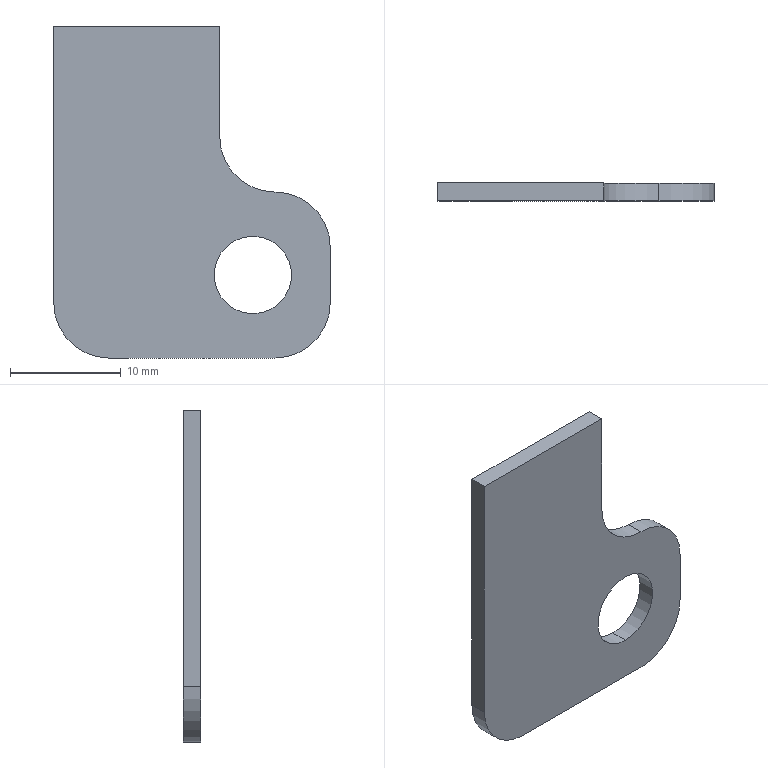Part | SolidWorks | features Fillet 1, FlatPattern 1, SMBaseFlange 1, SheetMetal 1 | 1 solid | 13 faces | box 25 x 1.6 x 30 mm | volume 881.257 mm3 | plane 7 | cylinder 6 | commonest cylinder face diameters 10 x4 7 x2
STEP:
#1=CARTESIAN_POINT('',(18.,-1.6,-26.));
#2=VERTEX_POINT('',#1);
#3=CARTESIAN_POINT('',(18.,-1.6,-19.));
#4=VERTEX_POINT('',#3);
#5=CARTESIAN_POINT('',(18.,-1.6,-22.5));
#6=DIRECTION('',(0.,1.,0.));
#7=DIRECTION('',(0.,0.,1.));
#8=AXIS2_PLACEMENT_3D('',#5,#6,#7);
#9=CIRCLE('',#8,3.5);
#10=EDGE_CURVE('',#2,#4,#9,.T.);
#11=ORIENTED_EDGE('',*,*,#10,.F.);
#12=CARTESIAN_POINT('',(18.,0.,-26.));
#13=VERTEX_POINT('',#12);
#14=CARTESIAN_POINT('',(18.,-1.6,-26.));
#15=DIRECTION('',(0.,1.,0.));
#16=VECTOR('',#15,1000.);
#17=LINE('',#14,#16);
#18=EDGE_CURVE('',#2,#13,#17,.T.);
#19=ORIENTED_EDGE('',*,*,#18,.T.);
#20=CARTESIAN_POINT('',(18.,0.,-19.));
#21=VERTEX_POINT('',#20);
#22=CARTESIAN_POINT('',(18.,0.,-22.5));
#23=DIRECTION('',(0.,1.,0.));
#24=DIRECTION('',(0.,0.,1.));
#25=AXIS2_PLACEMENT_3D('',#22,#23,#24);
#26=CIRCLE('',#25,3.5);
#27=EDGE_CURVE('',#13,#21,#26,.T.);
#28=ORIENTED_EDGE('',*,*,#27,.T.);
#29=CARTESIAN_POINT('',(18.,-1.6,-19.));
#30=DIRECTION('',(0.,1.,0.));
#31=VECTOR('',#30,1000.);
#32=LINE('',#29,#31);
#33=EDGE_CURVE('',#4,#21,#32,.T.);
#34=ORIENTED_EDGE('',*,*,#33,.F.);
#35=EDGE_LOOP('',(#11,#19,#28,#34));
#36=FACE_OUTER_BOUND('',#35,.T.);
#37=CARTESIAN_POINT('',(18.,-1.6,-22.5));
#38=DIRECTION('',(0.,1.,0.));
#39=DIRECTION('',(0.,0.,1.));
#40=AXIS2_PLACEMENT_3D('',#37,#38,#39);
#41=CYLINDRICAL_SURFACE('',#40,3.5);
#42=ADVANCED_FACE('',(#36),#41,.F.);
#43=CARTESIAN_POINT('',(0.,0.,-25.));
#44=VERTEX_POINT('',#43);
#45=CARTESIAN_POINT('',(0.,0.,0.));
#46=VERTEX_POINT('',#45);
#47=CARTESIAN_POINT('',(0.,0.,-30.));
#48=DIRECTION('',(0.,0.,1.));
#49=VECTOR('',#48,1000.);
#50=LINE('',#47,#49);
#51=EDGE_CURVE('',#44,#46,#50,.T.);
#52=ORIENTED_EDGE('',*,*,#51,.F.);
#53=CARTESIAN_POINT('',(0.,-1.6,-25.));
#54=VERTEX_POINT('',#53);
#55=CARTESIAN_POINT('',(0.,-1.6,-25.));
#56=DIRECTION('',(0.,-1.,0.));
#57=VECTOR('',#56,1000.);
#58=LINE('',#55,#57);
#59=EDGE_CURVE('',#44,#54,#58,.T.);
#60=ORIENTED_EDGE('',*,*,#59,.T.);
#61=CARTESIAN_POINT('',(0.,-1.6,0.));
#62=VERTEX_POINT('',#61);
#63=CARTESIAN_POINT('',(0.,-1.6,-30.));
#64=DIRECTION('',(0.,0.,1.));
#65=VECTOR('',#64,1000.);
#66=LINE('',#63,#65);
#67=EDGE_CURVE('',#54,#62,#66,.T.);
#68=ORIENTED_EDGE('',*,*,#67,.T.);
#69=CARTESIAN_POINT('',(0.,-1.6,0.));
#70=DIRECTION('',(0.,1.,0.));
#71=VECTOR('',#70,1000.);
#72=LINE('',#69,#71);
#73=EDGE_CURVE('',#62,#46,#72,.T.);
#74=ORIENTED_EDGE('',*,*,#73,.T.);
#75=EDGE_LOOP('',(#52,#60,#68,#74));
#76=FACE_OUTER_BOUND('',#75,.T.);
#77=CARTESIAN_POINT('',(0.,-1.6,-30.));
#78=DIRECTION('',(-1.,0.,0.));
#79=DIRECTION('',(0.,0.,1.));
#80=AXIS2_PLACEMENT_3D('',#77,#78,#79);
#81=PLANE('',#80);
#82=ADVANCED_FACE('',(#76),#81,.T.);
#83=CARTESIAN_POINT('',(20.,-1.6,-30.));
#84=VERTEX_POINT('',#83);
#85=CARTESIAN_POINT('',(5.,-1.6,-30.));
#86=VERTEX_POINT('',#85);
#87=CARTESIAN_POINT('',(25.,-1.6,-30.));
#88=DIRECTION('',(-1.,0.,0.));
#89=VECTOR('',#88,1000.);
#90=LINE('',#87,#89);
#91=EDGE_CURVE('',#84,#86,#90,.T.);
#92=ORIENTED_EDGE('',*,*,#91,.T.);
#93=CARTESIAN_POINT('',(5.,0.,-30.));
#94=VERTEX_POINT('',#93);
#95=CARTESIAN_POINT('',(5.,-1.6,-30.));
#96=DIRECTION('',(0.,1.,0.));
#97=VECTOR('',#96,1000.);
#98=LINE('',#95,#97);
#99=EDGE_CURVE('',#86,#94,#98,.T.);
#100=ORIENTED_EDGE('',*,*,#99,.T.);
#101=CARTESIAN_POINT('',(20.,0.,-30.));
#102=VERTEX_POINT('',#101);
#103=CARTESIAN_POINT('',(25.,0.,-30.));
#104=DIRECTION('',(-1.,0.,0.));
#105=VECTOR('',#104,1000.);
#106=LINE('',#103,#105);
#107=EDGE_CURVE('',#102,#94,#106,.T.);
#108=ORIENTED_EDGE('',*,*,#107,.F.);
#109=CARTESIAN_POINT('',(20.,-1.6,-30.));
#110=DIRECTION('',(0.,-1.,0.));
#111=VECTOR('',#110,1000.);
#112=LINE('',#109,#111);
#113=EDGE_CURVE('',#102,#84,#112,.T.);
#114=ORIENTED_EDGE('',*,*,#113,.T.);
#115=EDGE_LOOP('',(#92,#100,#108,#114));
#116=FACE_OUTER_BOUND('',#115,.T.);
#117=CARTESIAN_POINT('',(25.,-1.6,-30.));
#118=DIRECTION('',(0.,0.,-1.));
#119=DIRECTION('',(-1.,0.,0.));
#120=AXIS2_PLACEMENT_3D('',#117,#118,#119);
#121=PLANE('',#120);
#122=ADVANCED_FACE('',(#116),#121,.T.);
#123=CARTESIAN_POINT('',(25.,-1.6,-20.));
#124=VERTEX_POINT('',#123);
#125=CARTESIAN_POINT('',(25.,-1.6,-25.));
#126=VERTEX_POINT('',#125);
#127=CARTESIAN_POINT('',(25.,-1.6,-15.));
#128=DIRECTION('',(0.,0.,-1.));
#129=VECTOR('',#128,1000.);
#130=LINE('',#127,#129);
#131=EDGE_CURVE('',#124,#126,#130,.T.);
#132=ORIENTED_EDGE('',*,*,#131,.T.);
#133=CARTESIAN_POINT('',(25.,0.,-25.));
#134=VERTEX_POINT('',#133);
#135=CARTESIAN_POINT('',(25.,-1.6,-25.));
#136=DIRECTION('',(0.,1.,0.));
#137=VECTOR('',#136,1000.);
#138=LINE('',#135,#137);
#139=EDGE_CURVE('',#126,#134,#138,.T.);
#140=ORIENTED_EDGE('',*,*,#139,.T.);
#141=CARTESIAN_POINT('',(25.,0.,-20.));
#142=VERTEX_POINT('',#141);
#143=CARTESIAN_POINT('',(25.,0.,-15.));
#144=DIRECTION('',(0.,0.,-1.));
#145=VECTOR('',#144,1000.);
#146=LINE('',#143,#145);
#147=EDGE_CURVE('',#142,#134,#146,.T.);
#148=ORIENTED_EDGE('',*,*,#147,.F.);
#149=CARTESIAN_POINT('',(25.,-1.6,-20.));
#150=DIRECTION('',(0.,-1.,0.));
#151=VECTOR('',#150,1000.);
#152=LINE('',#149,#151);
#153=EDGE_CURVE('',#142,#124,#152,.T.);
#154=ORIENTED_EDGE('',*,*,#153,.T.);
#155=EDGE_LOOP('',(#132,#140,#148,#154));
#156=FACE_OUTER_BOUND('',#155,.T.);
#157=CARTESIAN_POINT('',(25.,-1.6,-15.));
#158=DIRECTION('',(1.,0.,0.));
#159=DIRECTION('',(0.,0.,-1.));
#160=AXIS2_PLACEMENT_3D('',#157,#158,#159);
#161=PLANE('',#160);
#162=ADVANCED_FACE('',(#156),#161,.T.);
#163=CARTESIAN_POINT('',(15.,-1.6,0.));
#164=VERTEX_POINT('',#163);
#165=CARTESIAN_POINT('',(15.,-1.6,-10.));
#166=VERTEX_POINT('',#165);
#167=CARTESIAN_POINT('',(15.,-1.6,0.));
#168=DIRECTION('',(0.,0.,-1.));
#169=VECTOR('',#168,1000.);
#170=LINE('',#167,#169);
#171=EDGE_CURVE('',#164,#166,#170,.T.);
#172=ORIENTED_EDGE('',*,*,#171,.T.);
#173=CARTESIAN_POINT('',(15.,0.,-10.));
#174=VERTEX_POINT('',#173);
#175=CARTESIAN_POINT('',(15.,0.,-10.));
#176=DIRECTION('',(0.,1.,0.));
#177=VECTOR('',#176,1000.);
#178=LINE('',#175,#177);
#179=EDGE_CURVE('',#166,#174,#178,.T.);
#180=ORIENTED_EDGE('',*,*,#179,.T.);
#181=CARTESIAN_POINT('',(15.,0.,0.));
#182=VERTEX_POINT('',#181);
#183=CARTESIAN_POINT('',(15.,0.,0.));
#184=DIRECTION('',(0.,0.,-1.));
#185=VECTOR('',#184,1000.);
#186=LINE('',#183,#185);
#187=EDGE_CURVE('',#182,#174,#186,.T.);
#188=ORIENTED_EDGE('',*,*,#187,.F.);
#189=CARTESIAN_POINT('',(15.,-1.6,0.));
#190=DIRECTION('',(0.,1.,0.));
#191=VECTOR('',#190,1000.);
#192=LINE('',#189,#191);
#193=EDGE_CURVE('',#164,#182,#192,.T.);
#194=ORIENTED_EDGE('',*,*,#193,.F.);
#195=EDGE_LOOP('',(#172,#180,#188,#194));
#196=FACE_OUTER_BOUND('',#195,.T.);
#197=CARTESIAN_POINT('',(15.,-1.6,0.));
#198=DIRECTION('',(1.,0.,0.));
#199=DIRECTION('',(0.,0.,-1.));
#200=AXIS2_PLACEMENT_3D('',#197,#198,#199);
#201=PLANE('',#200);
#202=ADVANCED_FACE('',(#196),#201,.T.);
#203=CARTESIAN_POINT('',(0.,0.,0.));
#204=DIRECTION('',(1.,0.,0.));
#205=VECTOR('',#204,1000.);
#206=LINE('',#203,#205);
#207=EDGE_CURVE('',#46,#182,#206,.T.);
#208=ORIENTED_EDGE('',*,*,#207,.F.);
#209=ORIENTED_EDGE('',*,*,#73,.F.);
#210=CARTESIAN_POINT('',(0.,-1.6,0.));
#211=DIRECTION('',(1.,0.,0.));
#212=VECTOR('',#211,1000.);
#213=LINE('',#210,#212);
#214=EDGE_CURVE('',#62,#164,#213,.T.);
#215=ORIENTED_EDGE('',*,*,#214,.T.);
#216=ORIENTED_EDGE('',*,*,#193,.T.);
#217=EDGE_LOOP('',(#208,#209,#215,#216));
#218=FACE_OUTER_BOUND('',#217,.T.);
#219=CARTESIAN_POINT('',(0.,-1.6,0.));
#220=DIRECTION('',(0.,0.,1.));
#221=DIRECTION('',(1.,0.,0.));
#222=AXIS2_PLACEMENT_3D('',#219,#220,#221);
#223=PLANE('',#222);
#224=ADVANCED_FACE('',(#218),#223,.T.);
#225=CARTESIAN_POINT('',(18.,-1.6,-22.5));
#226=DIRECTION('',(0.,1.,0.));
#227=DIRECTION('',(0.,0.,1.));
#228=AXIS2_PLACEMENT_3D('',#225,#226,#227);
#229=CIRCLE('',#228,3.5);
#230=EDGE_CURVE('',#4,#2,#229,.T.);
#231=ORIENTED_EDGE('',*,*,#230,.T.);
#232=ORIENTED_EDGE('',*,*,#10,.T.);
#233=EDGE_LOOP('',(#231,#232));
#234=FACE_BOUND('',#233,.T.);
#235=ORIENTED_EDGE('',*,*,#67,.F.);
#236=CARTESIAN_POINT('',(5.,-1.6,-25.));
#237=DIRECTION('',(0.,-1.,0.));
#238=DIRECTION('',(0.,0.,1.));
#239=AXIS2_PLACEMENT_3D('',#236,#237,#238);
#240=CIRCLE('',#239,5.);
#241=EDGE_CURVE('',#54,#86,#240,.T.);
#242=ORIENTED_EDGE('',*,*,#241,.T.);
#243=ORIENTED_EDGE('',*,*,#91,.F.);
#244=CARTESIAN_POINT('',(20.,-1.6,-25.));
#245=DIRECTION('',(0.,-1.,0.));
#246=DIRECTION('',(0.,0.,1.));
#247=AXIS2_PLACEMENT_3D('',#244,#245,#246);
#248=CIRCLE('',#247,5.);
#249=EDGE_CURVE('',#84,#126,#248,.T.);
#250=ORIENTED_EDGE('',*,*,#249,.T.);
#251=ORIENTED_EDGE('',*,*,#131,.F.);
#252=CARTESIAN_POINT('',(20.,-1.6,-15.));
#253=VERTEX_POINT('',#252);
#254=CARTESIAN_POINT('',(20.,-1.6,-20.));
#255=DIRECTION('',(0.,-1.,0.));
#256=DIRECTION('',(0.,0.,1.));
#257=AXIS2_PLACEMENT_3D('',#254,#255,#256);
#258=CIRCLE('',#257,5.);
#259=EDGE_CURVE('',#124,#253,#258,.T.);
#260=ORIENTED_EDGE('',*,*,#259,.T.);
#261=CARTESIAN_POINT('',(20.,-1.6,-10.));
#262=DIRECTION('',(0.,1.,0.));
#263=DIRECTION('',(0.,0.,1.));
#264=AXIS2_PLACEMENT_3D('',#261,#262,#263);
#265=CIRCLE('',#264,5.);
#266=EDGE_CURVE('',#253,#166,#265,.T.);
#267=ORIENTED_EDGE('',*,*,#266,.T.);
#268=ORIENTED_EDGE('',*,*,#171,.F.);
#269=ORIENTED_EDGE('',*,*,#214,.F.);
#270=EDGE_LOOP('',(#235,#242,#243,#250,#251,#260,#267,#268,#269));
#271=FACE_OUTER_BOUND('',#270,.T.);
#272=CARTESIAN_POINT('',(0.,-1.6,0.));
#273=DIRECTION('',(0.,1.,0.));
#274=DIRECTION('',(0.,0.,1.));
#275=AXIS2_PLACEMENT_3D('',#272,#273,#274);
#276=PLANE('',#275);
#277=ADVANCED_FACE('',(#234,#271),#276,.F.);
#278=CARTESIAN_POINT('',(18.,0.,-22.5));
#279=DIRECTION('',(0.,1.,0.));
#280=DIRECTION('',(0.,0.,1.));
#281=AXIS2_PLACEMENT_3D('',#278,#279,#280);
#282=CIRCLE('',#281,3.5);
#283=EDGE_CURVE('',#21,#13,#282,.T.);
#284=ORIENTED_EDGE('',*,*,#283,.F.);
#285=ORIENTED_EDGE('',*,*,#27,.F.);
#286=EDGE_LOOP('',(#284,#285));
#287=FACE_BOUND('',#286,.T.);
#288=ORIENTED_EDGE('',*,*,#107,.T.);
#289=CARTESIAN_POINT('',(5.,0.,-25.));
#290=DIRECTION('',(0.,1.,0.));
#291=DIRECTION('',(0.,0.,1.));
#292=AXIS2_PLACEMENT_3D('',#289,#290,#291);
#293=CIRCLE('',#292,5.);
#294=EDGE_CURVE('',#94,#44,#293,.T.);
#295=ORIENTED_EDGE('',*,*,#294,.T.);
#296=ORIENTED_EDGE('',*,*,#51,.T.);
#297=ORIENTED_EDGE('',*,*,#207,.T.);
#298=ORIENTED_EDGE('',*,*,#187,.T.);
#299=CARTESIAN_POINT('',(20.,0.,-15.));
#300=VERTEX_POINT('',#299);
#301=CARTESIAN_POINT('',(20.,0.,-10.));
#302=DIRECTION('',(0.,-1.,0.));
#303=DIRECTION('',(0.,0.,1.));
#304=AXIS2_PLACEMENT_3D('',#301,#302,#303);
#305=CIRCLE('',#304,5.);
#306=EDGE_CURVE('',#174,#300,#305,.T.);
#307=ORIENTED_EDGE('',*,*,#306,.T.);
#308=CARTESIAN_POINT('',(20.,0.,-20.));
#309=DIRECTION('',(0.,1.,0.));
#310=DIRECTION('',(0.,0.,1.));
#311=AXIS2_PLACEMENT_3D('',#308,#309,#310);
#312=CIRCLE('',#311,5.);
#313=EDGE_CURVE('',#300,#142,#312,.T.);
#314=ORIENTED_EDGE('',*,*,#313,.T.);
#315=ORIENTED_EDGE('',*,*,#147,.T.);
#316=CARTESIAN_POINT('',(20.,0.,-25.));
#317=DIRECTION('',(0.,1.,0.));
#318=DIRECTION('',(0.,0.,1.));
#319=AXIS2_PLACEMENT_3D('',#316,#317,#318);
#320=CIRCLE('',#319,5.);
#321=EDGE_CURVE('',#134,#102,#320,.T.);
#322=ORIENTED_EDGE('',*,*,#321,.T.);
#323=EDGE_LOOP('',(#288,#295,#296,#297,#298,#307,#314,#315,#322));
#324=FACE_OUTER_BOUND('',#323,.T.);
#325=CARTESIAN_POINT('',(0.,0.,0.));
#326=DIRECTION('',(0.,1.,0.));
#327=DIRECTION('',(0.,0.,1.));
#328=AXIS2_PLACEMENT_3D('',#325,#326,#327);
#329=PLANE('',#328);
#330=ADVANCED_FACE('',(#287,#324),#329,.T.);
#331=ORIENTED_EDGE('',*,*,#18,.F.);
#332=ORIENTED_EDGE('',*,*,#230,.F.);
#333=ORIENTED_EDGE('',*,*,#33,.T.);
#334=ORIENTED_EDGE('',*,*,#283,.T.);
#335=EDGE_LOOP('',(#331,#332,#333,#334));
#336=FACE_OUTER_BOUND('',#335,.T.);
#337=CARTESIAN_POINT('',(18.,-1.6,-22.5));
#338=DIRECTION('',(0.,1.,0.));
#339=DIRECTION('',(0.,0.,1.));
#340=AXIS2_PLACEMENT_3D('',#337,#338,#339);
#341=CYLINDRICAL_SURFACE('',#340,3.5);
#342=ADVANCED_FACE('',(#336),#341,.F.);
#343=ORIENTED_EDGE('',*,*,#241,.F.);
#344=ORIENTED_EDGE('',*,*,#59,.F.);
#345=ORIENTED_EDGE('',*,*,#294,.F.);
#346=ORIENTED_EDGE('',*,*,#99,.F.);
#347=EDGE_LOOP('',(#343,#344,#345,#346));
#348=FACE_OUTER_BOUND('',#347,.T.);
#349=CARTESIAN_POINT('',(5.,-1.6,-25.));
#350=DIRECTION('',(0.,1.,0.));
#351=DIRECTION('',(0.,0.,1.));
#352=AXIS2_PLACEMENT_3D('',#349,#350,#351);
#353=CYLINDRICAL_SURFACE('',#352,5.);
#354=ADVANCED_FACE('',(#348),#353,.T.);
#355=ORIENTED_EDGE('',*,*,#249,.F.);
#356=ORIENTED_EDGE('',*,*,#113,.F.);
#357=ORIENTED_EDGE('',*,*,#321,.F.);
#358=ORIENTED_EDGE('',*,*,#139,.F.);
#359=EDGE_LOOP('',(#355,#356,#357,#358));
#360=FACE_OUTER_BOUND('',#359,.T.);
#361=CARTESIAN_POINT('',(20.,-1.6,-25.));
#362=DIRECTION('',(0.,1.,0.));
#363=DIRECTION('',(0.,0.,1.));
#364=AXIS2_PLACEMENT_3D('',#361,#362,#363);
#365=CYLINDRICAL_SURFACE('',#364,5.);
#366=ADVANCED_FACE('',(#360),#365,.T.);
#367=ORIENTED_EDGE('',*,*,#179,.F.);
#368=ORIENTED_EDGE('',*,*,#266,.F.);
#369=CARTESIAN_POINT('',(20.,-1.6,-15.));
#370=DIRECTION('',(0.,-1.,0.));
#371=VECTOR('',#370,1000.);
#372=LINE('',#369,#371);
#373=EDGE_CURVE('',#300,#253,#372,.T.);
#374=ORIENTED_EDGE('',*,*,#373,.F.);
#375=ORIENTED_EDGE('',*,*,#306,.F.);
#376=EDGE_LOOP('',(#367,#368,#374,#375));
#377=FACE_OUTER_BOUND('',#376,.T.);
#378=CARTESIAN_POINT('',(20.,-1.6,-10.));
#379=DIRECTION('',(0.,-1.,0.));
#380=DIRECTION('',(0.,0.,-1.));
#381=AXIS2_PLACEMENT_3D('',#378,#379,#380);
#382=CYLINDRICAL_SURFACE('',#381,5.);
#383=ADVANCED_FACE('',(#377),#382,.F.);
#384=ORIENTED_EDGE('',*,*,#259,.F.);
#385=ORIENTED_EDGE('',*,*,#153,.F.);
#386=ORIENTED_EDGE('',*,*,#313,.F.);
#387=ORIENTED_EDGE('',*,*,#373,.T.);
#388=EDGE_LOOP('',(#384,#385,#386,#387));
#389=FACE_OUTER_BOUND('',#388,.T.);
#390=CARTESIAN_POINT('',(20.,-1.6,-20.));
#391=DIRECTION('',(0.,1.,0.));
#392=DIRECTION('',(0.,0.,1.));
#393=AXIS2_PLACEMENT_3D('',#390,#391,#392);
#394=CYLINDRICAL_SURFACE('',#393,5.);
#395=ADVANCED_FACE('',(#389),#394,.T.);
#396=CLOSED_SHELL('',(#42,#82,#122,#162,#202,#224,#277,#330,#342,#354,#366,#383,#395));
#397=MANIFOLD_SOLID_BREP('',#396);
#398=CARTESIAN_POINT('',(0.,0.,0.));
#399=DIRECTION('',(0.,0.,1.));
#400=DIRECTION('',(1.,0.,0.));
#401=AXIS2_PLACEMENT_3D('',#398,#399,#400);
#402=(LENGTH_UNIT()NAMED_UNIT(*)SI_UNIT(.MILLI.,.METRE.));
#403=UNCERTAINTY_MEASURE_WITH_UNIT(LENGTH_MEASURE(0.00001),#402,'','');
#404=(NAMED_UNIT(*)PLANE_ANGLE_UNIT()SI_UNIT($,.RADIAN.));
#405=(NAMED_UNIT(*)SI_UNIT($,.STERADIAN.)SOLID_ANGLE_UNIT());
#406=(GEOMETRIC_REPRESENTATION_CONTEXT(3)GLOBAL_UNCERTAINTY_ASSIGNED_CONTEXT((#403))GLOBAL_UNIT_ASSIGNED_CONTEXT((#402,#404,#405))REPRESENTATION_CONTEXT('',''));
#407=ADVANCED_BREP_SHAPE_REPRESENTATION('',(#397,#401),#406);